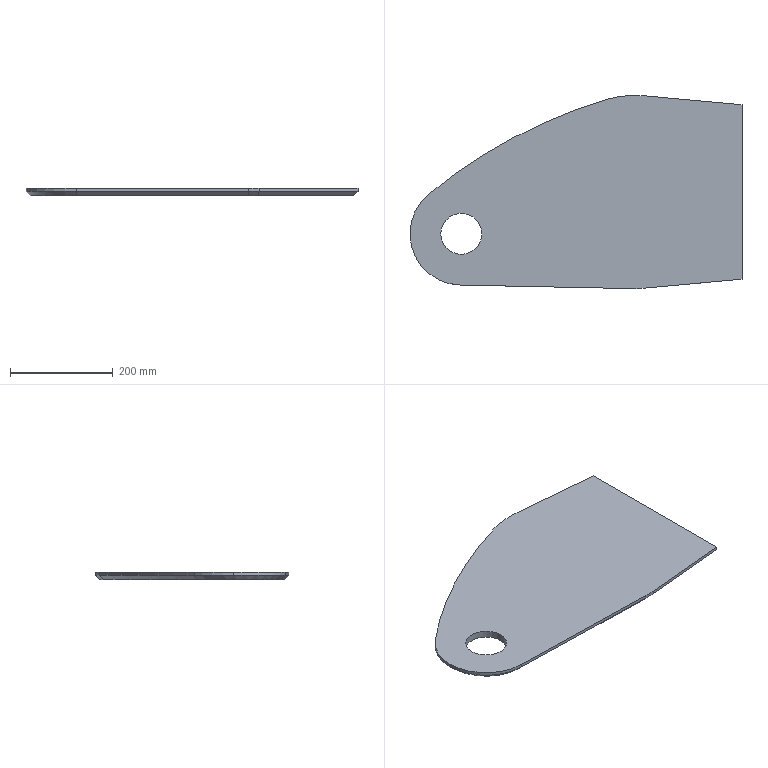Part | SolidWorks | features Chamfer 1, Extrusion 1 | 1 solid | 21 faces | box 647.5 x 377 x 14 mm | volume 2654377 mm3 | plane 10 | cylinder 7 | cone 4 | commonest cylinder face diameters 80 x2 200 x2 377 x2 2000 x1
STEP:
#1=CARTESIAN_POINT('',(-377.5,-81.6,14.));
#2=VERTEX_POINT('',#1);
#3=CARTESIAN_POINT('',(-297.5,-81.6,14.));
#4=VERTEX_POINT('',#3);
#5=CARTESIAN_POINT('',(-337.5,-81.6,14.));
#6=DIRECTION('',(0.,0.,1.));
#7=DIRECTION('',(1.,0.,0.));
#8=AXIS2_PLACEMENT_3D('',#5,#6,#7);
#9=CIRCLE('',#8,40.);
#10=EDGE_CURVE('',#2,#4,#9,.T.);
#11=ORIENTED_EDGE('',*,*,#10,.T.);
#12=CARTESIAN_POINT('',(-297.5,-81.6,0.));
#13=VERTEX_POINT('',#12);
#14=CARTESIAN_POINT('',(-297.5,-81.6,14.));
#15=DIRECTION('',(0.,0.,-1.));
#16=VECTOR('',#15,1000.);
#17=LINE('',#14,#16);
#18=EDGE_CURVE('',#4,#13,#17,.T.);
#19=ORIENTED_EDGE('',*,*,#18,.T.);
#20=CARTESIAN_POINT('',(-377.5,-81.6,0.));
#21=VERTEX_POINT('',#20);
#22=CARTESIAN_POINT('',(-337.5,-81.6,0.));
#23=DIRECTION('',(0.,0.,1.));
#24=DIRECTION('',(1.,0.,0.));
#25=AXIS2_PLACEMENT_3D('',#22,#23,#24);
#26=CIRCLE('',#25,40.);
#27=EDGE_CURVE('',#21,#13,#26,.T.);
#28=ORIENTED_EDGE('',*,*,#27,.F.);
#29=CARTESIAN_POINT('',(-377.5,-81.6,14.));
#30=DIRECTION('',(0.,0.,-1.));
#31=VECTOR('',#30,1000.);
#32=LINE('',#29,#31);
#33=EDGE_CURVE('',#2,#21,#32,.T.);
#34=ORIENTED_EDGE('',*,*,#33,.F.);
#35=EDGE_LOOP('',(#11,#19,#28,#34));
#36=FACE_OUTER_BOUND('',#35,.T.);
#37=CARTESIAN_POINT('',(-337.5,-81.6,14.));
#38=DIRECTION('',(0.,0.,-1.));
#39=DIRECTION('',(-1.,0.,0.));
#40=AXIS2_PLACEMENT_3D('',#37,#38,#39);
#41=CYLINDRICAL_SURFACE('',#40,40.);
#42=ADVANCED_FACE('',(#36),#41,.F.);
#43=CARTESIAN_POINT('',(-437.5,-81.6,14.));
#44=VERTEX_POINT('',#43);
#45=CARTESIAN_POINT('',(-339.55,-181.579,14.));
#46=VERTEX_POINT('',#45);
#47=CARTESIAN_POINT('',(-337.5,-81.6,14.));
#48=DIRECTION('',(0.,0.,1.));
#49=DIRECTION('',(1.,0.,0.));
#50=AXIS2_PLACEMENT_3D('',#47,#48,#49);
#51=CIRCLE('',#50,100.);
#52=EDGE_CURVE('',#44,#46,#51,.T.);
#53=ORIENTED_EDGE('',*,*,#52,.F.);
#54=CARTESIAN_POINT('',(-437.5,-81.6,8.));
#55=VERTEX_POINT('',#54);
#56=CARTESIAN_POINT('',(-437.5,-81.6,14.));
#57=DIRECTION('',(0.,0.,-1.));
#58=VECTOR('',#57,1000.);
#59=LINE('',#56,#58);
#60=EDGE_CURVE('',#44,#55,#59,.T.);
#61=ORIENTED_EDGE('',*,*,#60,.T.);
#62=CARTESIAN_POINT('',(-339.55,-181.579,8.));
#63=VERTEX_POINT('',#62);
#64=CARTESIAN_POINT('',(-337.5,-81.6,8.));
#65=DIRECTION('',(0.,0.,1.));
#66=DIRECTION('',(1.,0.,0.));
#67=AXIS2_PLACEMENT_3D('',#64,#65,#66);
#68=CIRCLE('',#67,100.);
#69=EDGE_CURVE('',#55,#63,#68,.T.);
#70=ORIENTED_EDGE('',*,*,#69,.T.);
#71=CARTESIAN_POINT('',(-339.55,-181.579,14.));
#72=DIRECTION('',(0.,0.,-1.));
#73=VECTOR('',#72,1000.);
#74=LINE('',#71,#73);
#75=EDGE_CURVE('',#46,#63,#74,.T.);
#76=ORIENTED_EDGE('',*,*,#75,.F.);
#77=EDGE_LOOP('',(#53,#61,#70,#76));
#78=FACE_OUTER_BOUND('',#77,.T.);
#79=CARTESIAN_POINT('',(-337.5,-81.6,14.));
#80=DIRECTION('',(0.,0.,-1.));
#81=DIRECTION('',(-1.,0.,0.));
#82=AXIS2_PLACEMENT_3D('',#79,#80,#81);
#83=CYLINDRICAL_SURFACE('',#82,100.);
#84=ADVANCED_FACE('',(#78),#83,.T.);
#85=CARTESIAN_POINT('',(-400.964,-4.319,14.));
#86=VERTEX_POINT('',#85);
#87=CARTESIAN_POINT('',(-337.5,-81.6,14.));
#88=DIRECTION('',(0.,0.,1.));
#89=DIRECTION('',(1.,0.,0.));
#90=AXIS2_PLACEMENT_3D('',#87,#88,#89);
#91=CIRCLE('',#90,100.);
#92=EDGE_CURVE('',#86,#44,#91,.T.);
#93=ORIENTED_EDGE('',*,*,#92,.T.);
#94=ORIENTED_EDGE('',*,*,#52,.T.);
#95=CARTESIAN_POINT('',(-3.863,-188.46,14.));
#96=VERTEX_POINT('',#95);
#97=CARTESIAN_POINT('',(-339.55,-181.579,14.));
#98=DIRECTION('',(0.9998,-0.0205,0.));
#99=VECTOR('',#98,1000.);
#100=LINE('',#97,#99);
#101=EDGE_CURVE('',#46,#96,#100,.T.);
#102=ORIENTED_EDGE('',*,*,#101,.T.);
#103=CARTESIAN_POINT('',(17.053,-187.727,14.));
#104=VERTEX_POINT('',#103);
#105=CARTESIAN_POINT('',(0.,0.,14.));
#106=DIRECTION('',(0.,0.,1.));
#107=DIRECTION('',(1.,0.,0.));
#108=AXIS2_PLACEMENT_3D('',#105,#106,#107);
#109=CIRCLE('',#108,188.5);
#110=EDGE_CURVE('',#96,#104,#109,.T.);
#111=ORIENTED_EDGE('',*,*,#110,.T.);
#112=CARTESIAN_POINT('',(210.,-170.2,14.));
#113=VERTEX_POINT('',#112);
#114=CARTESIAN_POINT('',(210.,-170.2,14.));
#115=DIRECTION('',(0.9959,0.09047,0.));
#116=VECTOR('',#115,1000.);
#117=LINE('',#114,#116);
#118=EDGE_CURVE('',#104,#113,#117,.T.);
#119=ORIENTED_EDGE('',*,*,#118,.T.);
#120=CARTESIAN_POINT('',(210.,170.2,14.));
#121=VERTEX_POINT('',#120);
#122=CARTESIAN_POINT('',(210.,170.2,14.));
#123=DIRECTION('',(0.,1.,0.));
#124=VECTOR('',#123,1000.);
#125=LINE('',#122,#124);
#126=EDGE_CURVE('',#113,#121,#125,.T.);
#127=ORIENTED_EDGE('',*,*,#126,.T.);
#128=CARTESIAN_POINT('',(17.053,187.727,14.));
#129=VERTEX_POINT('',#128);
#130=CARTESIAN_POINT('',(210.,170.2,14.));
#131=DIRECTION('',(-0.9959,0.09047,0.));
#132=VECTOR('',#131,1000.);
#133=LINE('',#130,#132);
#134=EDGE_CURVE('',#121,#129,#133,.T.);
#135=ORIENTED_EDGE('',*,*,#134,.T.);
#136=CARTESIAN_POINT('',(-54.279,180.516,14.));
#137=VERTEX_POINT('',#136);
#138=CARTESIAN_POINT('',(0.,0.,14.));
#139=DIRECTION('',(0.,0.,1.));
#140=DIRECTION('',(1.,0.,0.));
#141=AXIS2_PLACEMENT_3D('',#138,#139,#140);
#142=CIRCLE('',#141,188.5);
#143=EDGE_CURVE('',#129,#137,#142,.T.);
#144=ORIENTED_EDGE('',*,*,#143,.T.);
#145=CARTESIAN_POINT('',(233.674,-777.128,14.));
#146=DIRECTION('',(0.,0.,1.));
#147=DIRECTION('',(1.,0.,0.));
#148=AXIS2_PLACEMENT_3D('',#145,#146,#147);
#149=CIRCLE('',#148,1000.);
#150=EDGE_CURVE('',#137,#86,#149,.T.);
#151=ORIENTED_EDGE('',*,*,#150,.T.);
#152=EDGE_LOOP('',(#93,#94,#102,#111,#119,#127,#135,#144,#151));
#153=FACE_OUTER_BOUND('',#152,.T.);
#154=ORIENTED_EDGE('',*,*,#10,.F.);
#155=CARTESIAN_POINT('',(-337.5,-81.6,14.));
#156=DIRECTION('',(0.,0.,1.));
#157=DIRECTION('',(1.,0.,0.));
#158=AXIS2_PLACEMENT_3D('',#155,#156,#157);
#159=CIRCLE('',#158,40.);
#160=EDGE_CURVE('',#4,#2,#159,.T.);
#161=ORIENTED_EDGE('',*,*,#160,.F.);
#162=EDGE_LOOP('',(#154,#161));
#163=FACE_BOUND('',#162,.T.);
#164=CARTESIAN_POINT('',(-337.5,-81.6,14.));
#165=DIRECTION('',(0.,0.,1.));
#166=DIRECTION('',(1.,0.,0.));
#167=AXIS2_PLACEMENT_3D('',#164,#165,#166);
#168=PLANE('',#167);
#169=ADVANCED_FACE('',(#153,#163),#168,.T.);
#170=CARTESIAN_POINT('',(202.,-162.894,0.));
#171=VERTEX_POINT('',#170);
#172=CARTESIAN_POINT('',(16.329,-179.76,0.));
#173=VERTEX_POINT('',#172);
#174=CARTESIAN_POINT('',(-325.76,-210.835,0.));
#175=DIRECTION('',(-0.9959,-0.09047,0.));
#176=VECTOR('',#175,1000.);
#177=LINE('',#174,#176);
#178=EDGE_CURVE('',#171,#173,#177,.T.);
#179=ORIENTED_EDGE('',*,*,#178,.T.);
#180=CARTESIAN_POINT('',(-3.699,-180.462,0.));
#181=VERTEX_POINT('',#180);
#182=CARTESIAN_POINT('',(0.,0.,0.));
#183=DIRECTION('',(0.,0.,-1.));
#184=DIRECTION('',(1.,0.,0.));
#185=AXIS2_PLACEMENT_3D('',#182,#183,#184);
#186=CIRCLE('',#185,180.5);
#187=EDGE_CURVE('',#173,#181,#186,.T.);
#188=ORIENTED_EDGE('',*,*,#187,.T.);
#189=CARTESIAN_POINT('',(-339.386,-173.581,0.));
#190=VERTEX_POINT('',#189);
#191=CARTESIAN_POINT('',(-339.386,-173.581,0.));
#192=DIRECTION('',(-0.9998,0.0205,0.));
#193=VECTOR('',#192,1000.);
#194=LINE('',#191,#193);
#195=EDGE_CURVE('',#181,#190,#194,.T.);
#196=ORIENTED_EDGE('',*,*,#195,.T.);
#197=CARTESIAN_POINT('',(-395.887,-10.502,0.));
#198=VERTEX_POINT('',#197);
#199=CARTESIAN_POINT('',(-337.5,-81.6,0.));
#200=DIRECTION('',(0.,0.,-1.));
#201=DIRECTION('',(1.,0.,0.));
#202=AXIS2_PLACEMENT_3D('',#199,#200,#201);
#203=CIRCLE('',#202,92.);
#204=EDGE_CURVE('',#190,#198,#203,.T.);
#205=ORIENTED_EDGE('',*,*,#204,.T.);
#206=CARTESIAN_POINT('',(-51.976,172.855,0.));
#207=VERTEX_POINT('',#206);
#208=CARTESIAN_POINT('',(233.674,-777.128,0.));
#209=DIRECTION('',(0.,0.,-1.));
#210=DIRECTION('',(1.,0.,0.));
#211=AXIS2_PLACEMENT_3D('',#208,#209,#210);
#212=CIRCLE('',#211,992.);
#213=EDGE_CURVE('',#198,#207,#212,.T.);
#214=ORIENTED_EDGE('',*,*,#213,.T.);
#215=CARTESIAN_POINT('',(16.329,179.76,0.));
#216=VERTEX_POINT('',#215);
#217=CARTESIAN_POINT('',(0.,0.,0.));
#218=DIRECTION('',(0.,0.,-1.));
#219=DIRECTION('',(1.,0.,0.));
#220=AXIS2_PLACEMENT_3D('',#217,#218,#219);
#221=CIRCLE('',#220,180.5);
#222=EDGE_CURVE('',#207,#216,#221,.T.);
#223=ORIENTED_EDGE('',*,*,#222,.T.);
#224=CARTESIAN_POINT('',(202.,162.894,0.));
#225=VERTEX_POINT('',#224);
#226=CARTESIAN_POINT('',(-311.057,209.499,0.));
#227=DIRECTION('',(0.9959,-0.09047,0.));
#228=VECTOR('',#227,1000.);
#229=LINE('',#226,#228);
#230=EDGE_CURVE('',#216,#225,#229,.T.);
#231=ORIENTED_EDGE('',*,*,#230,.T.);
#232=CARTESIAN_POINT('',(202.,-81.6,0.));
#233=DIRECTION('',(0.,-1.,0.));
#234=VECTOR('',#233,1000.);
#235=LINE('',#232,#234);
#236=EDGE_CURVE('',#225,#171,#235,.T.);
#237=ORIENTED_EDGE('',*,*,#236,.T.);
#238=EDGE_LOOP('',(#179,#188,#196,#205,#214,#223,#231,#237));
#239=FACE_OUTER_BOUND('',#238,.T.);
#240=ORIENTED_EDGE('',*,*,#27,.T.);
#241=CARTESIAN_POINT('',(-337.5,-81.6,0.));
#242=DIRECTION('',(0.,0.,1.));
#243=DIRECTION('',(1.,0.,0.));
#244=AXIS2_PLACEMENT_3D('',#241,#242,#243);
#245=CIRCLE('',#244,40.);
#246=EDGE_CURVE('',#13,#21,#245,.T.);
#247=ORIENTED_EDGE('',*,*,#246,.T.);
#248=EDGE_LOOP('',(#240,#247));
#249=FACE_BOUND('',#248,.T.);
#250=CARTESIAN_POINT('',(-337.5,-81.6,0.));
#251=DIRECTION('',(0.,0.,1.));
#252=DIRECTION('',(1.,0.,0.));
#253=AXIS2_PLACEMENT_3D('',#250,#251,#252);
#254=PLANE('',#253);
#255=ADVANCED_FACE('',(#239,#249),#254,.F.);
#256=ORIENTED_EDGE('',*,*,#60,.F.);
#257=ORIENTED_EDGE('',*,*,#92,.F.);
#258=CARTESIAN_POINT('',(-400.964,-4.319,8.));
#259=VERTEX_POINT('',#258);
#260=CARTESIAN_POINT('',(-400.964,-4.319,14.));
#261=DIRECTION('',(0.,0.,-1.));
#262=VECTOR('',#261,1000.);
#263=LINE('',#260,#262);
#264=EDGE_CURVE('',#86,#259,#263,.T.);
#265=ORIENTED_EDGE('',*,*,#264,.T.);
#266=CARTESIAN_POINT('',(-337.5,-81.6,8.));
#267=DIRECTION('',(0.,0.,1.));
#268=DIRECTION('',(1.,0.,0.));
#269=AXIS2_PLACEMENT_3D('',#266,#267,#268);
#270=CIRCLE('',#269,100.);
#271=EDGE_CURVE('',#259,#55,#270,.T.);
#272=ORIENTED_EDGE('',*,*,#271,.T.);
#273=EDGE_LOOP('',(#256,#257,#265,#272));
#274=FACE_OUTER_BOUND('',#273,.T.);
#275=CARTESIAN_POINT('',(-337.5,-81.6,14.));
#276=DIRECTION('',(0.,0.,-1.));
#277=DIRECTION('',(-1.,0.,0.));
#278=AXIS2_PLACEMENT_3D('',#275,#276,#277);
#279=CYLINDRICAL_SURFACE('',#278,100.);
#280=ADVANCED_FACE('',(#274),#279,.T.);
#281=ORIENTED_EDGE('',*,*,#75,.T.);
#282=CARTESIAN_POINT('',(-3.863,-188.46,8.));
#283=VERTEX_POINT('',#282);
#284=CARTESIAN_POINT('',(-339.55,-181.579,8.));
#285=DIRECTION('',(0.9998,-0.0205,0.));
#286=VECTOR('',#285,1000.);
#287=LINE('',#284,#286);
#288=EDGE_CURVE('',#63,#283,#287,.T.);
#289=ORIENTED_EDGE('',*,*,#288,.T.);
#290=CARTESIAN_POINT('',(-3.863,-188.46,14.));
#291=DIRECTION('',(0.,0.,-1.));
#292=VECTOR('',#291,1000.);
#293=LINE('',#290,#292);
#294=EDGE_CURVE('',#96,#283,#293,.T.);
#295=ORIENTED_EDGE('',*,*,#294,.F.);
#296=ORIENTED_EDGE('',*,*,#101,.F.);
#297=EDGE_LOOP('',(#281,#289,#295,#296));
#298=FACE_OUTER_BOUND('',#297,.T.);
#299=CARTESIAN_POINT('',(-339.55,-181.579,14.));
#300=DIRECTION('',(0.0205,0.9998,0.));
#301=DIRECTION('',(-0.9998,0.0205,0.));
#302=AXIS2_PLACEMENT_3D('',#299,#300,#301);
#303=PLANE('',#302);
#304=ADVANCED_FACE('',(#298),#303,.F.);
#305=ORIENTED_EDGE('',*,*,#294,.T.);
#306=CARTESIAN_POINT('',(17.053,-187.727,8.));
#307=VERTEX_POINT('',#306);
#308=CARTESIAN_POINT('',(0.,0.,8.));
#309=DIRECTION('',(0.,0.,1.));
#310=DIRECTION('',(1.,0.,0.));
#311=AXIS2_PLACEMENT_3D('',#308,#309,#310);
#312=CIRCLE('',#311,188.5);
#313=EDGE_CURVE('',#283,#307,#312,.T.);
#314=ORIENTED_EDGE('',*,*,#313,.T.);
#315=CARTESIAN_POINT('',(17.053,-187.727,14.));
#316=DIRECTION('',(0.,0.,-1.));
#317=VECTOR('',#316,1000.);
#318=LINE('',#315,#317);
#319=EDGE_CURVE('',#104,#307,#318,.T.);
#320=ORIENTED_EDGE('',*,*,#319,.F.);
#321=ORIENTED_EDGE('',*,*,#110,.F.);
#322=EDGE_LOOP('',(#305,#314,#320,#321));
#323=FACE_OUTER_BOUND('',#322,.T.);
#324=CARTESIAN_POINT('',(0.,0.,14.));
#325=DIRECTION('',(0.,0.,-1.));
#326=DIRECTION('',(-1.,0.,0.));
#327=AXIS2_PLACEMENT_3D('',#324,#325,#326);
#328=CYLINDRICAL_SURFACE('',#327,188.5);
#329=ADVANCED_FACE('',(#323),#328,.T.);
#330=ORIENTED_EDGE('',*,*,#319,.T.);
#331=CARTESIAN_POINT('',(210.,-170.2,8.));
#332=VERTEX_POINT('',#331);
#333=CARTESIAN_POINT('',(210.,-170.2,8.));
#334=DIRECTION('',(0.9959,0.09047,0.));
#335=VECTOR('',#334,1000.);
#336=LINE('',#333,#335);
#337=EDGE_CURVE('',#307,#332,#336,.T.);
#338=ORIENTED_EDGE('',*,*,#337,.T.);
#339=CARTESIAN_POINT('',(210.,-170.2,14.));
#340=DIRECTION('',(0.,0.,-1.));
#341=VECTOR('',#340,1000.);
#342=LINE('',#339,#341);
#343=EDGE_CURVE('',#113,#332,#342,.T.);
#344=ORIENTED_EDGE('',*,*,#343,.F.);
#345=ORIENTED_EDGE('',*,*,#118,.F.);
#346=EDGE_LOOP('',(#330,#338,#344,#345));
#347=FACE_OUTER_BOUND('',#346,.T.);
#348=CARTESIAN_POINT('',(210.,-170.2,14.));
#349=DIRECTION('',(-0.09047,0.9959,0.));
#350=DIRECTION('',(-0.9959,-0.09047,0.));
#351=AXIS2_PLACEMENT_3D('',#348,#349,#350);
#352=PLANE('',#351);
#353=ADVANCED_FACE('',(#347),#352,.F.);
#354=ORIENTED_EDGE('',*,*,#343,.T.);
#355=CARTESIAN_POINT('',(210.,170.2,8.));
#356=VERTEX_POINT('',#355);
#357=CARTESIAN_POINT('',(210.,170.2,8.));
#358=DIRECTION('',(0.,1.,0.));
#359=VECTOR('',#358,1000.);
#360=LINE('',#357,#359);
#361=EDGE_CURVE('',#332,#356,#360,.T.);
#362=ORIENTED_EDGE('',*,*,#361,.T.);
#363=CARTESIAN_POINT('',(210.,170.2,14.));
#364=DIRECTION('',(0.,0.,-1.));
#365=VECTOR('',#364,1000.);
#366=LINE('',#363,#365);
#367=EDGE_CURVE('',#121,#356,#366,.T.);
#368=ORIENTED_EDGE('',*,*,#367,.F.);
#369=ORIENTED_EDGE('',*,*,#126,.F.);
#370=EDGE_LOOP('',(#354,#362,#368,#369));
#371=FACE_OUTER_BOUND('',#370,.T.);
#372=CARTESIAN_POINT('',(210.,170.2,14.));
#373=DIRECTION('',(-1.,0.,0.));
#374=DIRECTION('',(0.,-1.,0.));
#375=AXIS2_PLACEMENT_3D('',#372,#373,#374);
#376=PLANE('',#375);
#377=ADVANCED_FACE('',(#371),#376,.F.);
#378=ORIENTED_EDGE('',*,*,#367,.T.);
#379=CARTESIAN_POINT('',(17.053,187.727,8.));
#380=VERTEX_POINT('',#379);
#381=CARTESIAN_POINT('',(210.,170.2,8.));
#382=DIRECTION('',(-0.9959,0.09047,0.));
#383=VECTOR('',#382,1000.);
#384=LINE('',#381,#383);
#385=EDGE_CURVE('',#356,#380,#384,.T.);
#386=ORIENTED_EDGE('',*,*,#385,.T.);
#387=CARTESIAN_POINT('',(17.053,187.727,14.));
#388=DIRECTION('',(0.,0.,-1.));
#389=VECTOR('',#388,1000.);
#390=LINE('',#387,#389);
#391=EDGE_CURVE('',#129,#380,#390,.T.);
#392=ORIENTED_EDGE('',*,*,#391,.F.);
#393=ORIENTED_EDGE('',*,*,#134,.F.);
#394=EDGE_LOOP('',(#378,#386,#392,#393));
#395=FACE_OUTER_BOUND('',#394,.T.);
#396=CARTESIAN_POINT('',(210.,170.2,14.));
#397=DIRECTION('',(-0.09047,-0.9959,0.));
#398=DIRECTION('',(0.9959,-0.09047,0.));
#399=AXIS2_PLACEMENT_3D('',#396,#397,#398);
#400=PLANE('',#399);
#401=ADVANCED_FACE('',(#395),#400,.F.);
#402=ORIENTED_EDGE('',*,*,#391,.T.);
#403=CARTESIAN_POINT('',(-54.279,180.516,8.));
#404=VERTEX_POINT('',#403);
#405=CARTESIAN_POINT('',(0.,0.,8.));
#406=DIRECTION('',(0.,0.,1.));
#407=DIRECTION('',(1.,0.,0.));
#408=AXIS2_PLACEMENT_3D('',#405,#406,#407);
#409=CIRCLE('',#408,188.5);
#410=EDGE_CURVE('',#380,#404,#409,.T.);
#411=ORIENTED_EDGE('',*,*,#410,.T.);
#412=CARTESIAN_POINT('',(-54.279,180.516,14.));
#413=DIRECTION('',(0.,0.,-1.));
#414=VECTOR('',#413,1000.);
#415=LINE('',#412,#414);
#416=EDGE_CURVE('',#137,#404,#415,.T.);
#417=ORIENTED_EDGE('',*,*,#416,.F.);
#418=ORIENTED_EDGE('',*,*,#143,.F.);
#419=EDGE_LOOP('',(#402,#411,#417,#418));
#420=FACE_OUTER_BOUND('',#419,.T.);
#421=CARTESIAN_POINT('',(0.,0.,14.));
#422=DIRECTION('',(0.,0.,-1.));
#423=DIRECTION('',(-1.,0.,0.));
#424=AXIS2_PLACEMENT_3D('',#421,#422,#423);
#425=CYLINDRICAL_SURFACE('',#424,188.5);
#426=ADVANCED_FACE('',(#420),#425,.T.);
#427=ORIENTED_EDGE('',*,*,#416,.T.);
#428=CARTESIAN_POINT('',(233.674,-777.128,8.));
#429=DIRECTION('',(0.,0.,1.));
#430=DIRECTION('',(1.,0.,0.));
#431=AXIS2_PLACEMENT_3D('',#428,#429,#430);
#432=CIRCLE('',#431,1000.);
#433=EDGE_CURVE('',#404,#259,#432,.T.);
#434=ORIENTED_EDGE('',*,*,#433,.T.);
#435=ORIENTED_EDGE('',*,*,#264,.F.);
#436=ORIENTED_EDGE('',*,*,#150,.F.);
#437=EDGE_LOOP('',(#427,#434,#435,#436));
#438=FACE_OUTER_BOUND('',#437,.T.);
#439=CARTESIAN_POINT('',(233.674,-777.128,14.));
#440=DIRECTION('',(0.,0.,-1.));
#441=DIRECTION('',(-1.,0.,0.));
#442=AXIS2_PLACEMENT_3D('',#439,#440,#441);
#443=CYLINDRICAL_SURFACE('',#442,1000.);
#444=ADVANCED_FACE('',(#438),#443,.T.);
#445=ORIENTED_EDGE('',*,*,#18,.F.);
#446=ORIENTED_EDGE('',*,*,#160,.T.);
#447=ORIENTED_EDGE('',*,*,#33,.T.);
#448=ORIENTED_EDGE('',*,*,#246,.F.);
#449=EDGE_LOOP('',(#445,#446,#447,#448));
#450=FACE_OUTER_BOUND('',#449,.T.);
#451=CARTESIAN_POINT('',(-337.5,-81.6,14.));
#452=DIRECTION('',(0.,0.,-1.));
#453=DIRECTION('',(-1.,0.,0.));
#454=AXIS2_PLACEMENT_3D('',#451,#452,#453);
#455=CYLINDRICAL_SURFACE('',#454,40.);
#456=ADVANCED_FACE('',(#450),#455,.F.);
#457=CARTESIAN_POINT('',(16.329,179.76,0.));
#458=DIRECTION('',(0.06397,0.7042,0.7071));
#459=VECTOR('',#458,1000.);
#460=LINE('',#457,#459);
#461=EDGE_CURVE('',#216,#380,#460,.T.);
#462=ORIENTED_EDGE('',*,*,#461,.F.);
#463=ORIENTED_EDGE('',*,*,#222,.F.);
#464=CARTESIAN_POINT('',(-54.279,180.516,8.));
#465=DIRECTION('',(0.2036,-0.6772,-0.7071));
#466=VECTOR('',#465,1000.);
#467=LINE('',#464,#466);
#468=EDGE_CURVE('',#404,#207,#467,.T.);
#469=ORIENTED_EDGE('',*,*,#468,.F.);
#470=ORIENTED_EDGE('',*,*,#410,.F.);
#471=EDGE_LOOP('',(#462,#463,#469,#470));
#472=FACE_OUTER_BOUND('',#471,.T.);
#473=CARTESIAN_POINT('',(0.,0.,8.));
#474=DIRECTION('',(0.,0.,1.));
#475=DIRECTION('',(1.,0.,0.));
#476=AXIS2_PLACEMENT_3D('',#473,#474,#475);
#477=CONICAL_SURFACE('',#476,188.5,0.7854);
#478=ADVANCED_FACE('',(#472),#477,.T.);
#479=ORIENTED_EDGE('',*,*,#468,.T.);
#480=ORIENTED_EDGE('',*,*,#213,.F.);
#481=CARTESIAN_POINT('',(-400.964,-4.319,8.));
#482=DIRECTION('',(0.4488,-0.5465,-0.7071));
#483=VECTOR('',#482,1000.);
#484=LINE('',#481,#483);
#485=EDGE_CURVE('',#259,#198,#484,.T.);
#486=ORIENTED_EDGE('',*,*,#485,.F.);
#487=ORIENTED_EDGE('',*,*,#433,.F.);
#488=EDGE_LOOP('',(#479,#480,#486,#487));
#489=FACE_OUTER_BOUND('',#488,.T.);
#490=CARTESIAN_POINT('',(233.674,-777.128,8.));
#491=DIRECTION('',(0.,0.,1.));
#492=DIRECTION('',(1.,0.,0.));
#493=AXIS2_PLACEMENT_3D('',#490,#491,#492);
#494=CONICAL_SURFACE('',#493,1000.,0.7854);
#495=ADVANCED_FACE('',(#489),#494,.T.);
#496=ORIENTED_EDGE('',*,*,#461,.T.);
#497=ORIENTED_EDGE('',*,*,#385,.F.);
#498=CARTESIAN_POINT('',(210.,170.2,8.));
#499=DIRECTION('',(0.594,0.5425,0.594));
#500=VECTOR('',#499,1000.);
#501=LINE('',#498,#500);
#502=EDGE_CURVE('',#225,#356,#501,.T.);
#503=ORIENTED_EDGE('',*,*,#502,.F.);
#504=ORIENTED_EDGE('',*,*,#230,.F.);
#505=EDGE_LOOP('',(#496,#497,#503,#504));
#506=FACE_OUTER_BOUND('',#505,.T.);
#507=CARTESIAN_POINT('',(210.,170.2,8.));
#508=DIRECTION('',(-0.06397,-0.7042,0.7071));
#509=DIRECTION('',(0.,-0.7086,-0.7057));
#510=AXIS2_PLACEMENT_3D('',#507,#508,#509);
#511=PLANE('',#510);
#512=ADVANCED_FACE('',(#506),#511,.F.);
#513=ORIENTED_EDGE('',*,*,#485,.T.);
#514=ORIENTED_EDGE('',*,*,#204,.F.);
#515=CARTESIAN_POINT('',(-339.55,-181.579,8.));
#516=DIRECTION('',(0.01449,0.707,-0.7071));
#517=VECTOR('',#516,1000.);
#518=LINE('',#515,#517);
#519=EDGE_CURVE('',#63,#190,#518,.T.);
#520=ORIENTED_EDGE('',*,*,#519,.F.);
#521=ORIENTED_EDGE('',*,*,#69,.F.);
#522=ORIENTED_EDGE('',*,*,#271,.F.);
#523=EDGE_LOOP('',(#513,#514,#520,#521,#522));
#524=FACE_OUTER_BOUND('',#523,.T.);
#525=CARTESIAN_POINT('',(-337.5,-81.6,8.));
#526=DIRECTION('',(0.,0.,1.));
#527=DIRECTION('',(1.,0.,0.));
#528=AXIS2_PLACEMENT_3D('',#525,#526,#527);
#529=CONICAL_SURFACE('',#528,100.,0.7854);
#530=ADVANCED_FACE('',(#524),#529,.T.);
#531=ORIENTED_EDGE('',*,*,#502,.T.);
#532=ORIENTED_EDGE('',*,*,#361,.F.);
#533=CARTESIAN_POINT('',(100.306,-70.019,-101.694));
#534=DIRECTION('',(0.594,-0.5425,0.594));
#535=VECTOR('',#534,1000.);
#536=LINE('',#533,#535);
#537=EDGE_CURVE('',#171,#332,#536,.T.);
#538=ORIENTED_EDGE('',*,*,#537,.F.);
#539=ORIENTED_EDGE('',*,*,#236,.F.);
#540=EDGE_LOOP('',(#531,#532,#538,#539));
#541=FACE_OUTER_BOUND('',#540,.T.);
#542=CARTESIAN_POINT('',(210.,170.2,8.));
#543=DIRECTION('',(-0.7071,0.,0.7071));
#544=DIRECTION('',(0.7071,0.,0.7071));
#545=AXIS2_PLACEMENT_3D('',#542,#543,#544);
#546=PLANE('',#545);
#547=ADVANCED_FACE('',(#541),#546,.F.);
#548=ORIENTED_EDGE('',*,*,#519,.T.);
#549=ORIENTED_EDGE('',*,*,#195,.F.);
#550=CARTESIAN_POINT('',(-3.863,-188.46,8.));
#551=DIRECTION('',(0.01449,0.707,-0.7071));
#552=VECTOR('',#551,1000.);
#553=LINE('',#550,#552);
#554=EDGE_CURVE('',#283,#181,#553,.T.);
#555=ORIENTED_EDGE('',*,*,#554,.F.);
#556=ORIENTED_EDGE('',*,*,#288,.F.);
#557=EDGE_LOOP('',(#548,#549,#555,#556));
#558=FACE_OUTER_BOUND('',#557,.T.);
#559=CARTESIAN_POINT('',(-339.55,-181.579,8.));
#560=DIRECTION('',(0.01449,0.707,0.7071));
#561=DIRECTION('',(0.,-0.7072,0.707));
#562=AXIS2_PLACEMENT_3D('',#559,#560,#561);
#563=PLANE('',#562);
#564=ADVANCED_FACE('',(#558),#563,.F.);
#565=ORIENTED_EDGE('',*,*,#537,.T.);
#566=ORIENTED_EDGE('',*,*,#337,.F.);
#567=CARTESIAN_POINT('',(16.329,-179.76,0.));
#568=DIRECTION('',(0.06397,-0.7042,0.7071));
#569=VECTOR('',#568,1000.);
#570=LINE('',#567,#569);
#571=EDGE_CURVE('',#173,#307,#570,.T.);
#572=ORIENTED_EDGE('',*,*,#571,.F.);
#573=ORIENTED_EDGE('',*,*,#178,.F.);
#574=EDGE_LOOP('',(#565,#566,#572,#573));
#575=FACE_OUTER_BOUND('',#574,.T.);
#576=CARTESIAN_POINT('',(210.,-170.2,8.));
#577=DIRECTION('',(-0.06397,0.7042,0.7071));
#578=DIRECTION('',(0.,-0.7086,0.7057));
#579=AXIS2_PLACEMENT_3D('',#576,#577,#578);
#580=PLANE('',#579);
#581=ADVANCED_FACE('',(#575),#580,.F.);
#582=ORIENTED_EDGE('',*,*,#554,.T.);
#583=ORIENTED_EDGE('',*,*,#187,.F.);
#584=ORIENTED_EDGE('',*,*,#571,.T.);
#585=ORIENTED_EDGE('',*,*,#313,.F.);
#586=EDGE_LOOP('',(#582,#583,#584,#585));
#587=FACE_OUTER_BOUND('',#586,.T.);
#588=CARTESIAN_POINT('',(0.,0.,8.));
#589=DIRECTION('',(0.,0.,1.));
#590=DIRECTION('',(1.,0.,0.));
#591=AXIS2_PLACEMENT_3D('',#588,#589,#590);
#592=CONICAL_SURFACE('',#591,188.5,0.7854);
#593=ADVANCED_FACE('',(#587),#592,.T.);
#594=CLOSED_SHELL('',(#42,#84,#169,#255,#280,#304,#329,#353,#377,#401,#426,#444,#456,#478,#495,#512,#530,#547,#564,#581,#593));
#595=MANIFOLD_SOLID_BREP('',#594);
#596=CARTESIAN_POINT('',(0.,0.,0.));
#597=DIRECTION('',(0.,0.,1.));
#598=DIRECTION('',(1.,0.,0.));
#599=AXIS2_PLACEMENT_3D('',#596,#597,#598);
#600=(LENGTH_UNIT()NAMED_UNIT(*)SI_UNIT(.MILLI.,.METRE.));
#601=UNCERTAINTY_MEASURE_WITH_UNIT(LENGTH_MEASURE(0.00001),#600,'','');
#602=(NAMED_UNIT(*)PLANE_ANGLE_UNIT()SI_UNIT($,.RADIAN.));
#603=(NAMED_UNIT(*)SI_UNIT($,.STERADIAN.)SOLID_ANGLE_UNIT());
#604=(GEOMETRIC_REPRESENTATION_CONTEXT(3)GLOBAL_UNCERTAINTY_ASSIGNED_CONTEXT((#601))GLOBAL_UNIT_ASSIGNED_CONTEXT((#600,#602,#603))REPRESENTATION_CONTEXT('',''));
#605=ADVANCED_BREP_SHAPE_REPRESENTATION('',(#595,#599),#604);